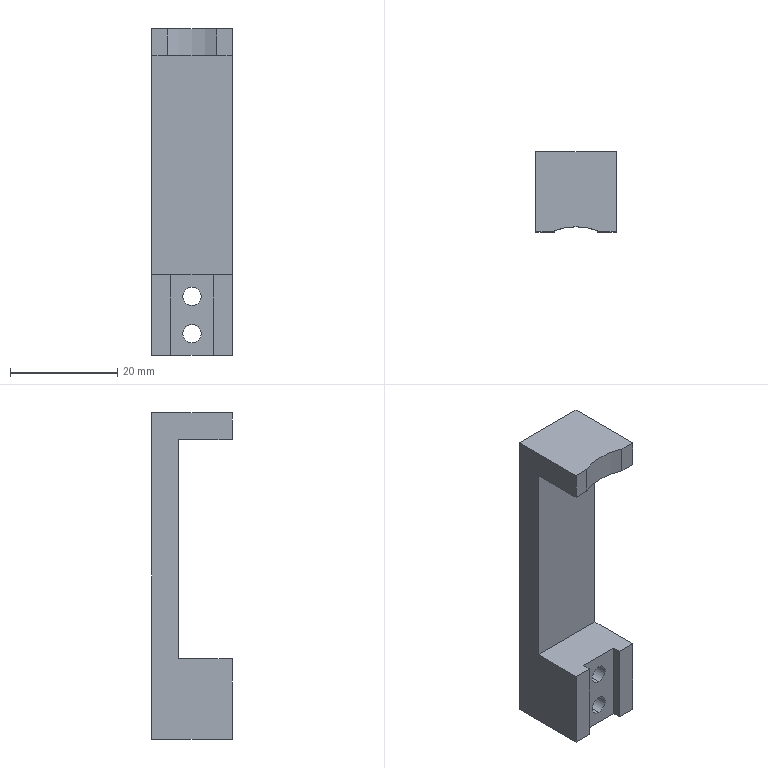Part | STEP file | PN_0045 | 1 solid | 26 faces | box 15 x 15 x 61 mm | volume 6956 mm3 | plane 17 | cylinder 9 | commonest cylinder face diameters 3.4 x4 6.5 x4 23.5 x1